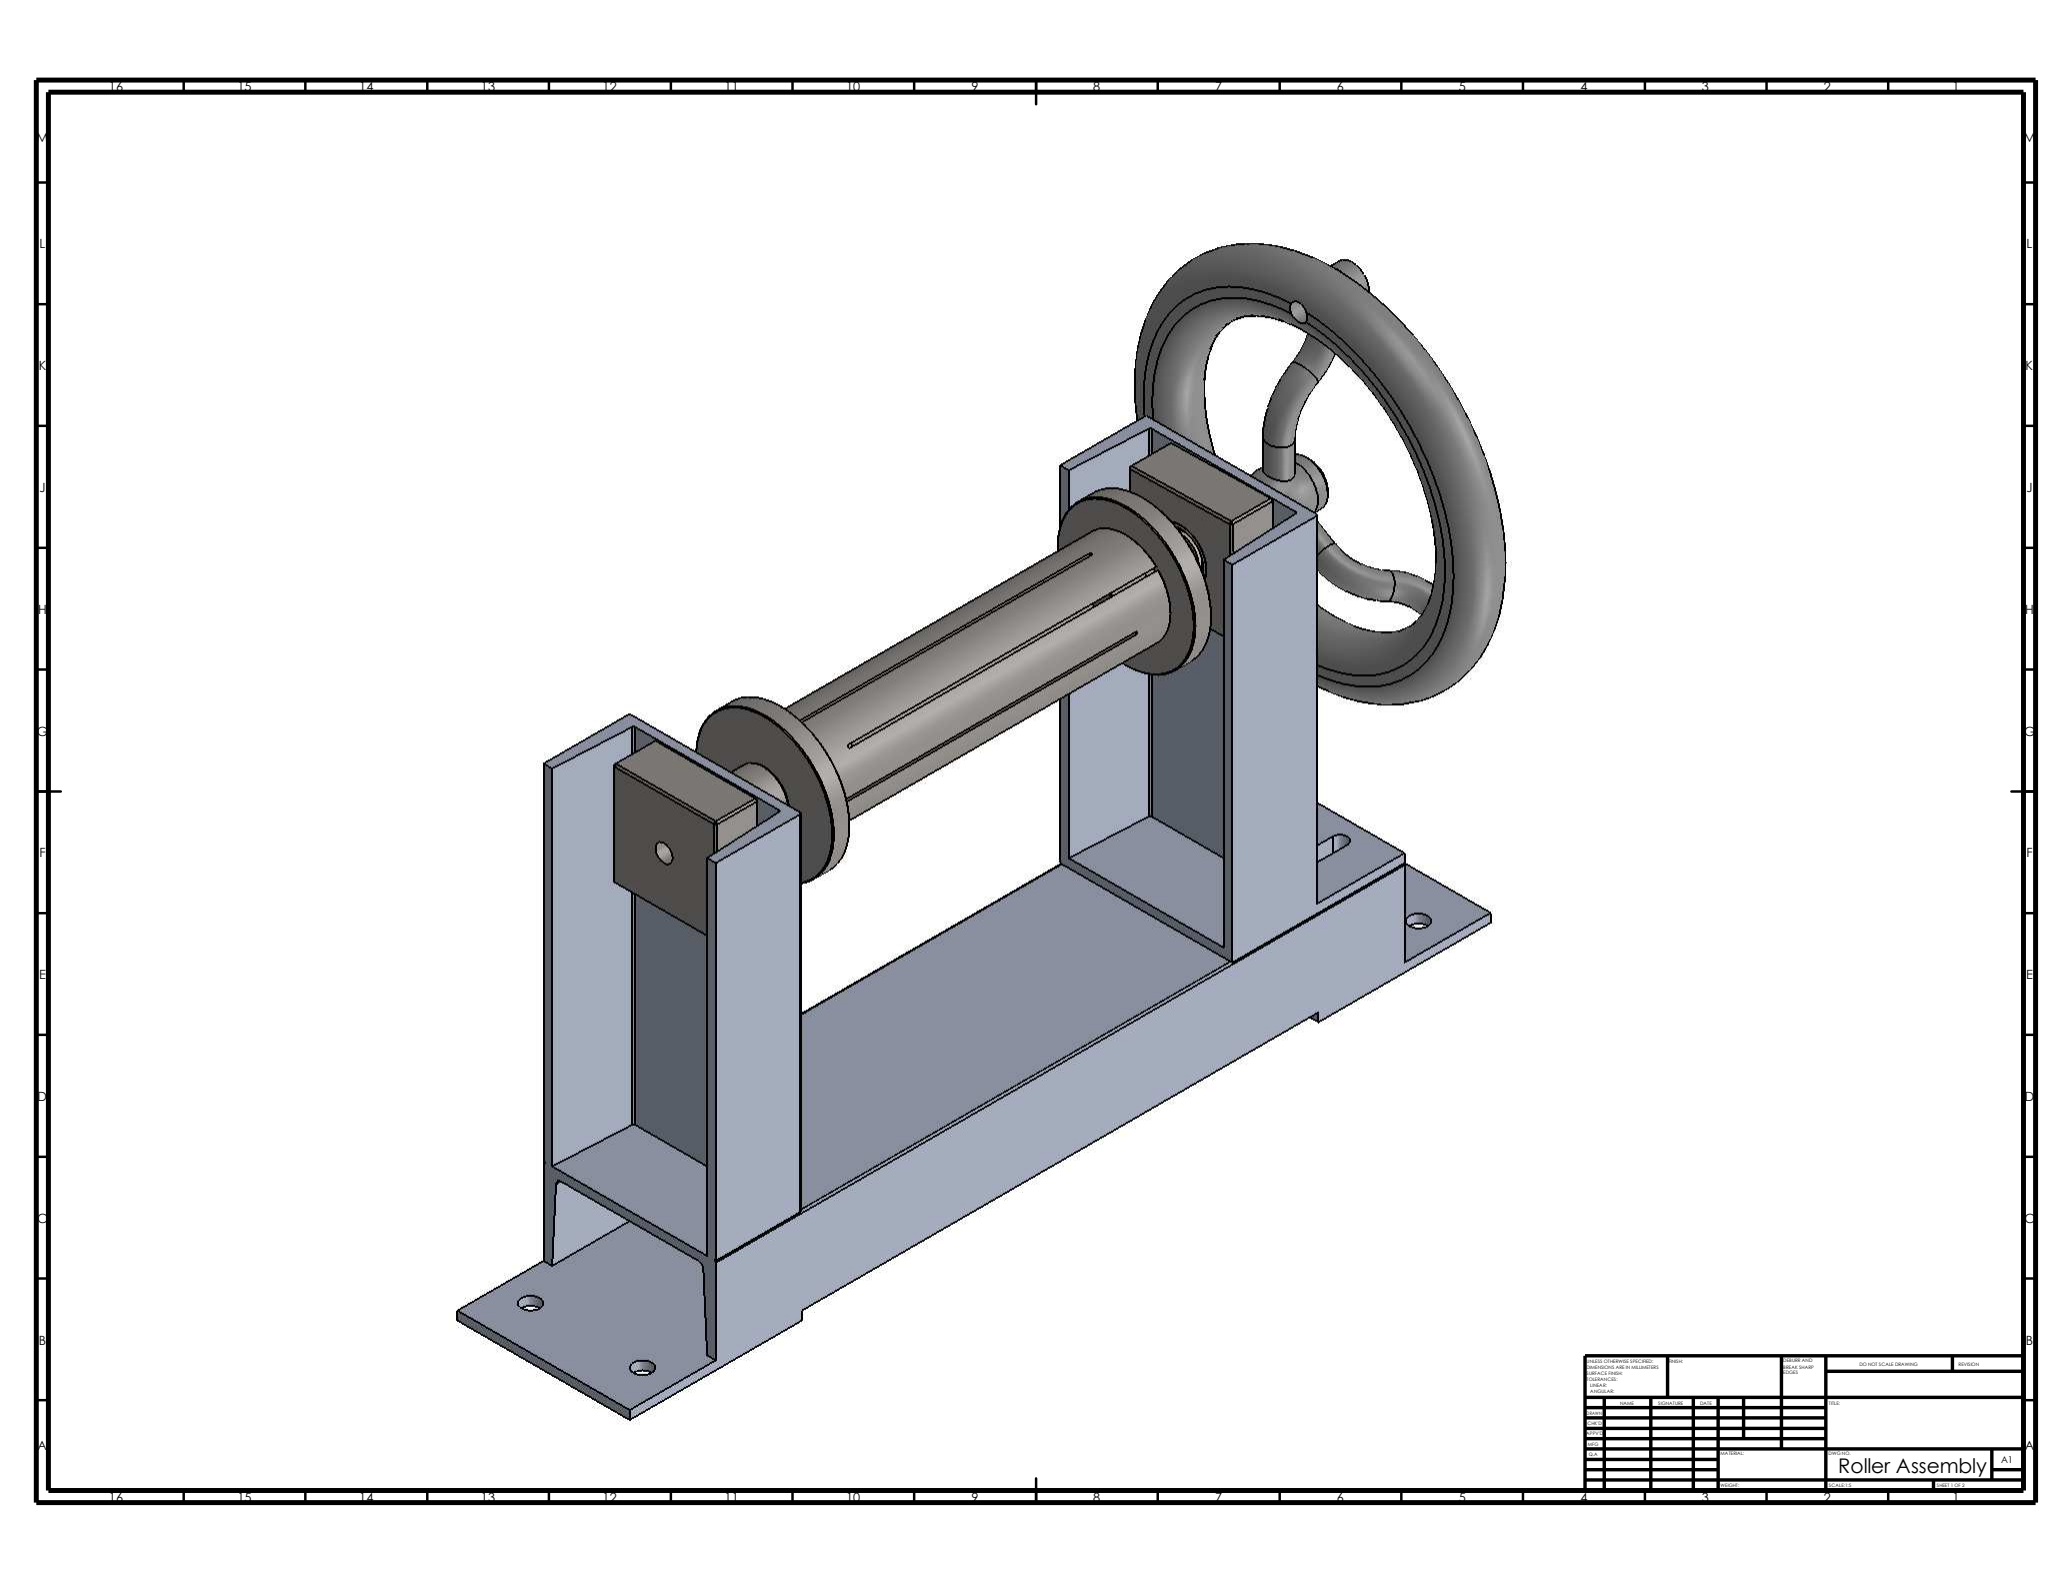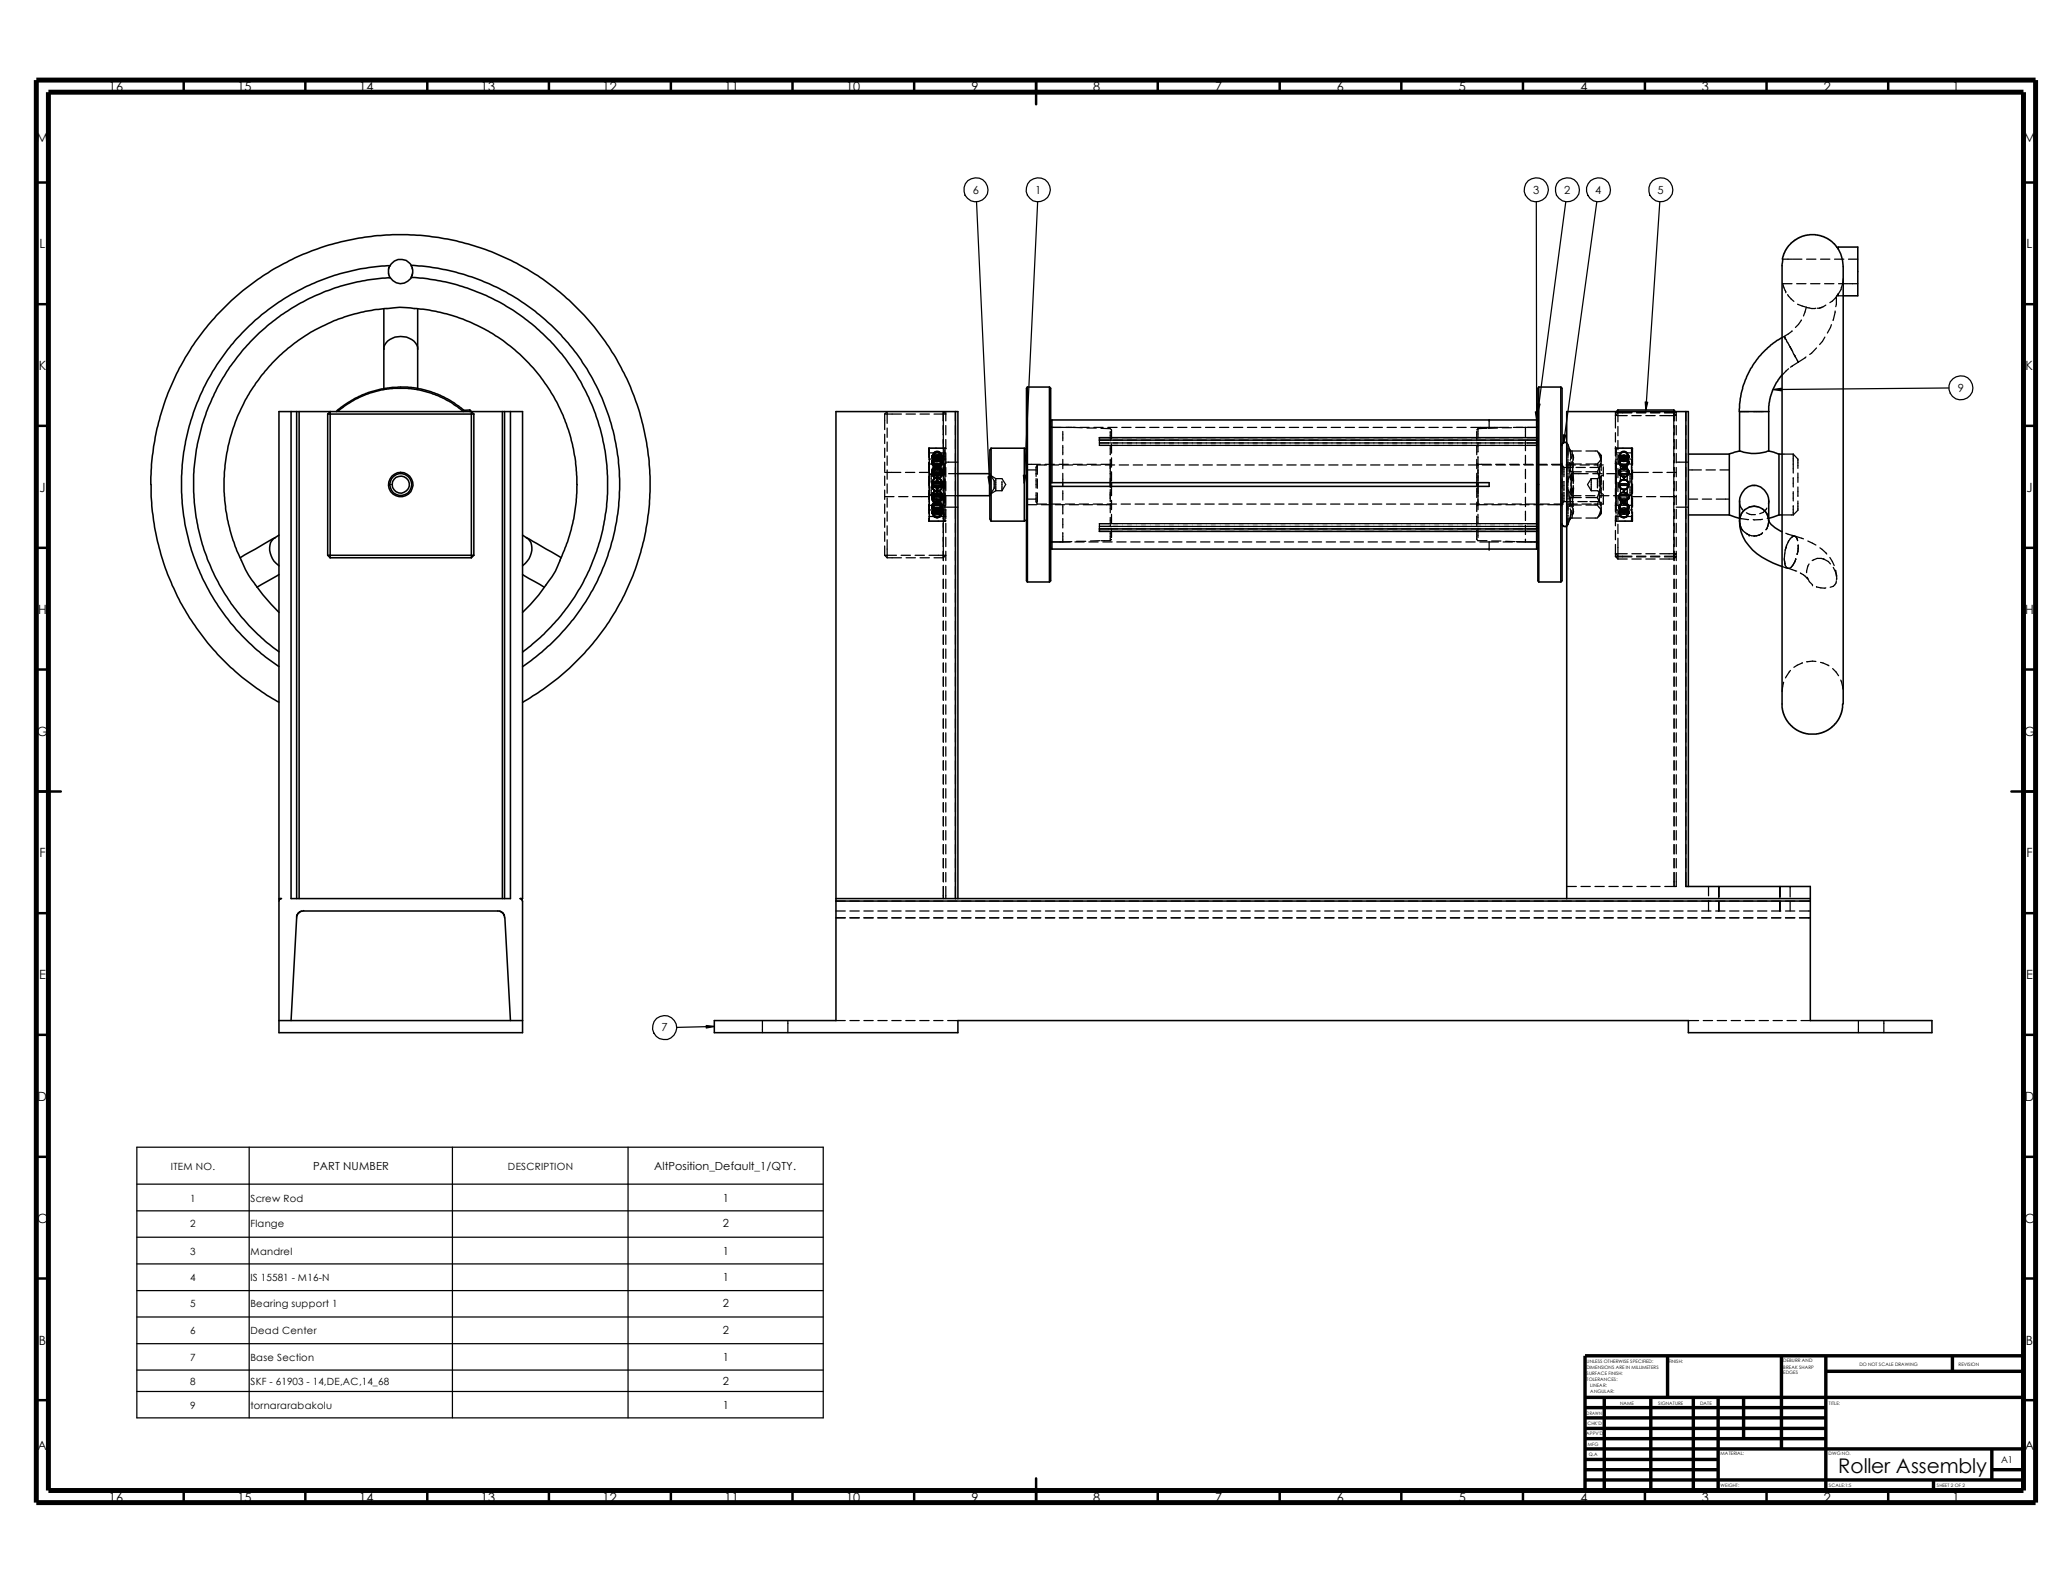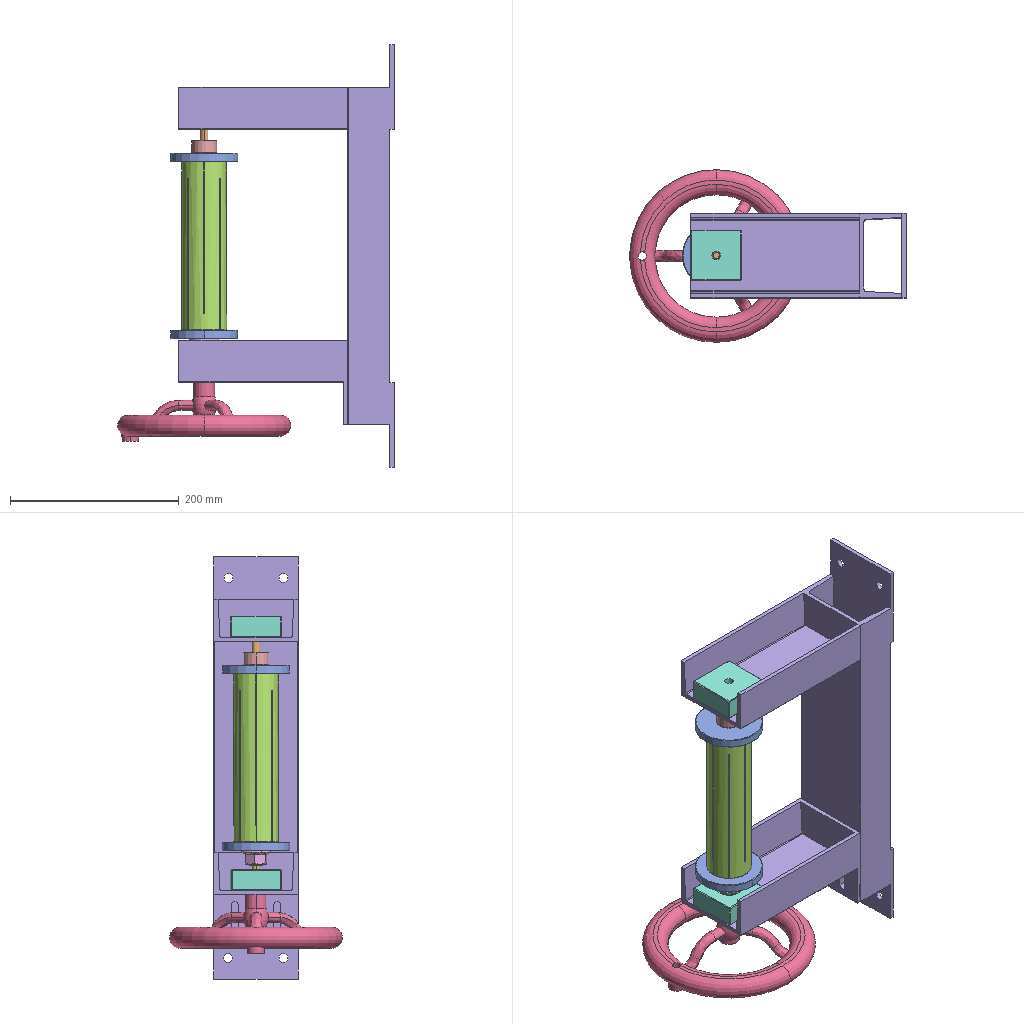Assembly | SolidWorks | 10 different items | 13 placed | box 327 x 205 x 500 mm
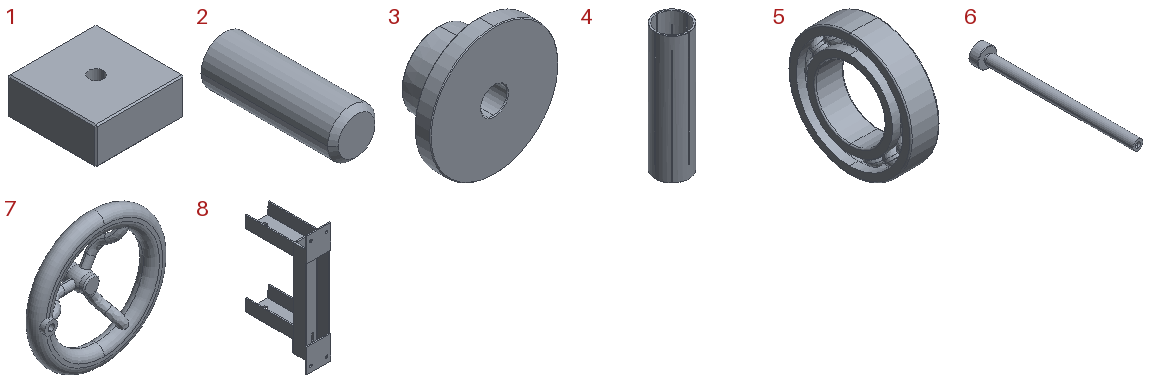Parts list (item | name | quantity | size | volume | features):
1 | - | x2 | 60 x 60 x 25 mm | 83354 mm3 | features ICE 2, Chamfer 1, Extrusion 1
2 | - | x2 | 9 x 26.875 x 9 mm | 1635 mm3 | features Chamfer 1, Revolution 1
3 | - | x2 | 80 x 35 x 80 mm | 85328 mm3 | features Chamfer 1, Revolution 1
4 | - | x1 | 53 x 53 x 200 mm | 87700 mm3 | features ICE 3, CirPattern 2, Chamfer 1, Extrusion 1, RefAxis 1
5 | - | x1 | 7 x 30 x 30 mm | 2289 mm3 | features Revolution 6, Attribute 3, CirPattern 2, RevCut 2, RefAxis 1
6 | - | x1 | 30 x 252 x 30 mm | 57567 mm3 | features Chamfer 3, HoleWzd 2, Revolution 1
7 | - | x1 | 205 x 69.5 x 205 mm | 388207 mm3 | features ICE 3, Revolution 2, CirPattern 1, Sweep 1
8 | - | x1 | 100 x 255 x 500 mm | 980990 mm3 | features ICE 5, HoleWzd 2, Extrusion 1
9 | hexagon flange nut_is | x1 | - | - | -
10 | radial ball bearing_68_skf | x1 | - | - | -
Mates (type | each side: item.copy, entity, surface, feature):
Concentric | 6.1 face cylinder Revolve1 | 3.1 face cylinder Revolve1
Coincident | 6.1 face plane Revolve1 | 3.1 face plane Revolve1
Concentric | 3.1 face cylinder Revolve1 | 4.1 face cylinder Cut-Extrude1
Coincident | 3.1 face plane Revolve1 | 4.1 face plane Boss-Extrude1
Concentric | 6.1 face cylinder Revolve1 | 3.2 face cylinder Revolve1
Coincident | 4.1 face plane Boss-Extrude1 | 3.2 face plane Revolve1
Concentric | 1.1 face cylinder Cut-Extrude2 | 2.1 face cylinder Revolve1
Coincident | 1.1 face plane Cut-Extrude1 | 2.1 face plane Revolve1
Concentric | 1.2 face cylinder Cut-Extrude2 | 2.2 face cylinder Revolve1
Coincident | 1.2 face plane Cut-Extrude1 | 2.2 face plane Revolve1
Concentric | 6.1 face cone Chamfer1 | 2.2 face cone Revolve1
Concentric | 6.1 face cone Chamfer3 | 2.1 face cone Revolve1
Coincident | 1.2 face plane Boss-Extrude1 | 8.1 face plane Boss-Extrude5
Concentric | 1.2 face cylinder Cut-Extrude2 | 8.1 face cylinder Ø18.5 (18.5) Diameter Hole1
Coincident | 1.1 face plane Boss-Extrude1 | 8.1 face plane Boss-Extrude3
Concentric | 8.1 face cylinder Ø18.5 (18.5) Diameter Hole1 | 7.1 face cylinder Cut-Extrude1
Coincident | 8.1 face plane Boss-Extrude5 | 7.1 face plane Revolve1